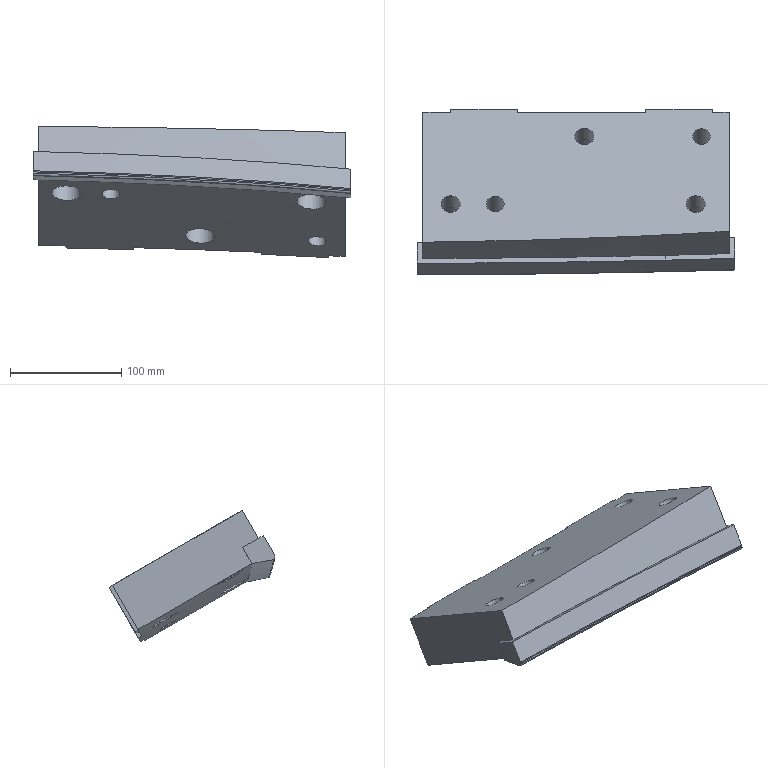Part | NX | features MAIN_BODY 2 | 1 solid | 38 faces | box 285 x 148.907 x 117.874 mm | volume 1791574 mm3 | plane 20 | spline 10 | cylinder 8 | commonest cylinder face diameters 17 x3 26 x3 16 x2